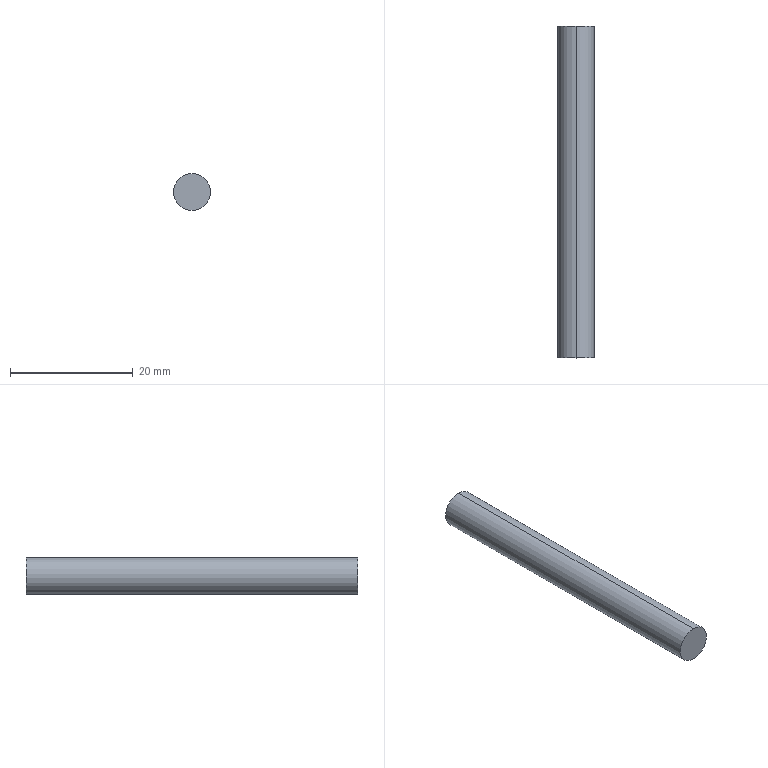Part | STEP file | Hinge shaft | 1 solid | 4 faces | box 6 x 54 x 6 mm | volume 1527 mm3 | cylinder 2 | plane 2 | commonest cylinder face diameters 6 x2
STEP:
#1=CARTESIAN_POINT('',(0.,0.,0.));
#2=DIRECTION('',(0.,0.,1.));
#3=DIRECTION('',(1.,0.,0.));
#4=AXIS2_PLACEMENT_3D('',#1,#2,#3);
#5=CARTESIAN_POINT('',(0.,54.,-3.));
#6=VERTEX_POINT('',#5);
#7=CARTESIAN_POINT('',(0.,54.,3.));
#8=VERTEX_POINT('',#7);
#9=CARTESIAN_POINT('',(0.,54.,0.));
#10=DIRECTION('',(0.,-1.,0.));
#11=DIRECTION('',(0.,0.,-1.));
#12=AXIS2_PLACEMENT_3D('',#9,#10,#11);
#13=CIRCLE('',#12,3.);
#14=CARTESIAN_POINT('',(0.,54.,0.));
#15=DIRECTION('',(0.,-1.,0.));
#16=DIRECTION('',(0.,0.,-1.));
#17=AXIS2_PLACEMENT_3D('',#14,#15,#16);
#18=CYLINDRICAL_SURFACE('',#17,3.);
#19=CARTESIAN_POINT('',(0.,0.));
#20=DIRECTION('',(1.,0.));
#21=VECTOR('',#20,1.);
#22=LINE('',#19,#21);
#23=(GEOMETRIC_REPRESENTATION_CONTEXT(2)PARAMETRIC_REPRESENTATION_CONTEXT()REPRESENTATION_CONTEXT('',''));
#24=DEFINITIONAL_REPRESENTATION('',(#22),#23);
#25=PCURVE('',#18,#24);
#26=CARTESIAN_POINT('',(0.,54.,0.));
#27=DIRECTION('',(0.,1.,0.));
#28=DIRECTION('',(0.,0.,1.));
#29=AXIS2_PLACEMENT_3D('',#26,#27,#28);
#30=PLANE('',#29);
#31=CARTESIAN_POINT('',(-3.,0.));
#32=CARTESIAN_POINT('',(-3.,5.196));
#33=CARTESIAN_POINT('',(1.5,2.598));
#34=CARTESIAN_POINT('',(6.,0.));
#35=CARTESIAN_POINT('',(1.5,-2.598));
#36=CARTESIAN_POINT('',(-3.,-5.196));
#37=CARTESIAN_POINT('',(-3.,0.));
#38=(BOUNDED_CURVE()B_SPLINE_CURVE(2,(#31,#32,#33,#34,#35,#36,#37),.UNSPECIFIED.,.T.,.F.)B_SPLINE_CURVE_WITH_KNOTS((1,2,2,2,2,1),(-2.094,0.,2.094,4.189,6.283,8.378),.UNSPECIFIED.)CURVE()GEOMETRIC_REPRESENTATION_ITEM()RATIONAL_B_SPLINE_CURVE((1.,0.5,1.,0.5,1.,0.5,1.))REPRESENTATION_ITEM(''));
#39=(GEOMETRIC_REPRESENTATION_CONTEXT(2)PARAMETRIC_REPRESENTATION_CONTEXT()REPRESENTATION_CONTEXT('',''));
#40=DEFINITIONAL_REPRESENTATION('',(#38),#39);
#41=PCURVE('',#30,#40);
#42=SURFACE_CURVE('',#13,(#25,#41),.PCURVE_S1.);
#43=EDGE_CURVE('',#6,#8,#42,.T.);
#44=ORIENTED_EDGE('',*,*,#43,.T.);
#45=CARTESIAN_POINT('',(0.,0.,3.));
#46=VERTEX_POINT('',#45);
#47=CARTESIAN_POINT('',(0.,54.,3.));
#48=DIRECTION('',(0.,-1.,0.));
#49=VECTOR('',#48,1.);
#50=LINE('',#47,#49);
#51=CARTESIAN_POINT('',(3.142,0.));
#52=DIRECTION('',(0.,1.));
#53=VECTOR('',#52,1.);
#54=LINE('',#51,#53);
#55=(GEOMETRIC_REPRESENTATION_CONTEXT(2)PARAMETRIC_REPRESENTATION_CONTEXT()REPRESENTATION_CONTEXT('',''));
#56=DEFINITIONAL_REPRESENTATION('',(#54),#55);
#57=PCURVE('',#18,#56);
#58=CARTESIAN_POINT('',(0.,54.,0.));
#59=DIRECTION('',(0.,-1.,0.));
#60=DIRECTION('',(0.,0.,-1.));
#61=AXIS2_PLACEMENT_3D('',#58,#59,#60);
#62=CYLINDRICAL_SURFACE('',#61,3.);
#63=CARTESIAN_POINT('',(3.142,0.));
#64=DIRECTION('',(0.,1.));
#65=VECTOR('',#64,1.);
#66=LINE('',#63,#65);
#67=(GEOMETRIC_REPRESENTATION_CONTEXT(2)PARAMETRIC_REPRESENTATION_CONTEXT()REPRESENTATION_CONTEXT('',''));
#68=DEFINITIONAL_REPRESENTATION('',(#66),#67);
#69=PCURVE('',#62,#68);
#70=SURFACE_CURVE('',#50,(#57,#69),.PCURVE_S1.);
#71=EDGE_CURVE('',#8,#46,#70,.T.);
#72=ORIENTED_EDGE('',*,*,#71,.T.);
#73=CARTESIAN_POINT('',(0.,0.,-3.));
#74=VERTEX_POINT('',#73);
#75=CARTESIAN_POINT('',(0.,0.,0.));
#76=DIRECTION('',(0.,1.,0.));
#77=DIRECTION('',(0.,0.,-1.));
#78=AXIS2_PLACEMENT_3D('',#75,#76,#77);
#79=CIRCLE('',#78,3.);
#80=CARTESIAN_POINT('',(6.283,54.));
#81=DIRECTION('',(-1.,0.));
#82=VECTOR('',#81,1.);
#83=LINE('',#80,#82);
#84=(GEOMETRIC_REPRESENTATION_CONTEXT(2)PARAMETRIC_REPRESENTATION_CONTEXT()REPRESENTATION_CONTEXT('',''));
#85=DEFINITIONAL_REPRESENTATION('',(#83),#84);
#86=PCURVE('',#18,#85);
#87=CARTESIAN_POINT('',(0.,0.,0.));
#88=DIRECTION('',(0.,1.,0.));
#89=DIRECTION('',(0.,0.,1.));
#90=AXIS2_PLACEMENT_3D('',#87,#88,#89);
#91=PLANE('',#90);
#92=CARTESIAN_POINT('',(0.,0.));
#93=DIRECTION('',(-1.,0.));
#94=AXIS2_PLACEMENT_2D('',#92,#93);
#95=CIRCLE('',#94,3.);
#96=(GEOMETRIC_REPRESENTATION_CONTEXT(2)PARAMETRIC_REPRESENTATION_CONTEXT()REPRESENTATION_CONTEXT('',''));
#97=DEFINITIONAL_REPRESENTATION('',(#95),#96);
#98=PCURVE('',#91,#97);
#99=SURFACE_CURVE('',#79,(#86,#98),.PCURVE_S1.);
#100=EDGE_CURVE('',#46,#74,#99,.T.);
#101=ORIENTED_EDGE('',*,*,#100,.T.);
#102=CARTESIAN_POINT('',(0.,54.,-3.));
#103=DIRECTION('',(0.,-1.,0.));
#104=VECTOR('',#103,1.);
#105=LINE('',#102,#104);
#106=CARTESIAN_POINT('',(0.,0.));
#107=DIRECTION('',(0.,1.));
#108=VECTOR('',#107,1.);
#109=LINE('',#106,#108);
#110=(GEOMETRIC_REPRESENTATION_CONTEXT(2)PARAMETRIC_REPRESENTATION_CONTEXT()REPRESENTATION_CONTEXT('',''));
#111=DEFINITIONAL_REPRESENTATION('',(#109),#110);
#112=PCURVE('',#18,#111);
#113=CARTESIAN_POINT('',(6.283,0.));
#114=DIRECTION('',(0.,1.));
#115=VECTOR('',#114,1.);
#116=LINE('',#113,#115);
#117=(GEOMETRIC_REPRESENTATION_CONTEXT(2)PARAMETRIC_REPRESENTATION_CONTEXT()REPRESENTATION_CONTEXT('',''));
#118=DEFINITIONAL_REPRESENTATION('',(#116),#117);
#119=PCURVE('',#62,#118);
#120=SURFACE_CURVE('',#105,(#112,#119),.PCURVE_S1.);
#121=EDGE_CURVE('',#6,#74,#120,.T.);
#122=ORIENTED_EDGE('',*,*,#121,.F.);
#123=EDGE_LOOP('',(#44,#72,#101,#122));
#124=FACE_BOUND('',#123,.T.);
#125=ADVANCED_FACE('',(#124),#18,.T.);
#126=ORIENTED_EDGE('',*,*,#71,.F.);
#127=CARTESIAN_POINT('',(0.,54.,0.));
#128=DIRECTION('',(0.,-1.,0.));
#129=DIRECTION('',(0.,0.,-1.));
#130=AXIS2_PLACEMENT_3D('',#127,#128,#129);
#131=CIRCLE('',#130,3.);
#132=CARTESIAN_POINT('',(0.,0.));
#133=DIRECTION('',(1.,0.));
#134=VECTOR('',#133,1.);
#135=LINE('',#132,#134);
#136=(GEOMETRIC_REPRESENTATION_CONTEXT(2)PARAMETRIC_REPRESENTATION_CONTEXT()REPRESENTATION_CONTEXT('',''));
#137=DEFINITIONAL_REPRESENTATION('',(#135),#136);
#138=PCURVE('',#62,#137);
#139=CARTESIAN_POINT('',(-3.,0.));
#140=CARTESIAN_POINT('',(-3.,5.196));
#141=CARTESIAN_POINT('',(1.5,2.598));
#142=CARTESIAN_POINT('',(6.,0.));
#143=CARTESIAN_POINT('',(1.5,-2.598));
#144=CARTESIAN_POINT('',(-3.,-5.196));
#145=CARTESIAN_POINT('',(-3.,0.));
#146=(BOUNDED_CURVE()B_SPLINE_CURVE(2,(#139,#140,#141,#142,#143,#144,#145),.UNSPECIFIED.,.T.,.F.)B_SPLINE_CURVE_WITH_KNOTS((1,2,2,2,2,1),(-2.094,0.,2.094,4.189,6.283,8.378),.UNSPECIFIED.)CURVE()GEOMETRIC_REPRESENTATION_ITEM()RATIONAL_B_SPLINE_CURVE((1.,0.5,1.,0.5,1.,0.5,1.))REPRESENTATION_ITEM(''));
#147=(GEOMETRIC_REPRESENTATION_CONTEXT(2)PARAMETRIC_REPRESENTATION_CONTEXT()REPRESENTATION_CONTEXT('',''));
#148=DEFINITIONAL_REPRESENTATION('',(#146),#147);
#149=PCURVE('',#30,#148);
#150=SURFACE_CURVE('',#131,(#138,#149),.PCURVE_S1.);
#151=EDGE_CURVE('',#8,#6,#150,.T.);
#152=ORIENTED_EDGE('',*,*,#151,.T.);
#153=ORIENTED_EDGE('',*,*,#121,.T.);
#154=CARTESIAN_POINT('',(0.,0.,0.));
#155=DIRECTION('',(0.,1.,0.));
#156=DIRECTION('',(0.,0.,-1.));
#157=AXIS2_PLACEMENT_3D('',#154,#155,#156);
#158=CIRCLE('',#157,3.);
#159=CARTESIAN_POINT('',(6.283,54.));
#160=DIRECTION('',(-1.,0.));
#161=VECTOR('',#160,1.);
#162=LINE('',#159,#161);
#163=(GEOMETRIC_REPRESENTATION_CONTEXT(2)PARAMETRIC_REPRESENTATION_CONTEXT()REPRESENTATION_CONTEXT('',''));
#164=DEFINITIONAL_REPRESENTATION('',(#162),#163);
#165=PCURVE('',#62,#164);
#166=CARTESIAN_POINT('',(0.,0.));
#167=DIRECTION('',(-1.,0.));
#168=AXIS2_PLACEMENT_2D('',#166,#167);
#169=CIRCLE('',#168,3.);
#170=(GEOMETRIC_REPRESENTATION_CONTEXT(2)PARAMETRIC_REPRESENTATION_CONTEXT()REPRESENTATION_CONTEXT('',''));
#171=DEFINITIONAL_REPRESENTATION('',(#169),#170);
#172=PCURVE('',#91,#171);
#173=SURFACE_CURVE('',#158,(#165,#172),.PCURVE_S1.);
#174=EDGE_CURVE('',#74,#46,#173,.T.);
#175=ORIENTED_EDGE('',*,*,#174,.T.);
#176=EDGE_LOOP('',(#126,#152,#153,#175));
#177=FACE_BOUND('',#176,.T.);
#178=ADVANCED_FACE('',(#177),#62,.T.);
#179=ORIENTED_EDGE('',*,*,#174,.F.);
#180=ORIENTED_EDGE('',*,*,#100,.F.);
#181=EDGE_LOOP('',(#179,#180));
#182=FACE_BOUND('',#181,.T.);
#183=ADVANCED_FACE('',(#182),#91,.F.);
#184=ORIENTED_EDGE('',*,*,#43,.F.);
#185=ORIENTED_EDGE('',*,*,#151,.F.);
#186=EDGE_LOOP('',(#184,#185));
#187=FACE_BOUND('',#186,.T.);
#188=ADVANCED_FACE('',(#187),#30,.T.);
#189=CLOSED_SHELL('',(#125,#178,#183,#188));
#190=MANIFOLD_SOLID_BREP('',#189);
#191=(LENGTH_UNIT()NAMED_UNIT(*)SI_UNIT(.MILLI.,.METRE.));
#192=UNCERTAINTY_MEASURE_WITH_UNIT(LENGTH_MEASURE(0.0000001),#191,'','');
#193=(NAMED_UNIT(*)PLANE_ANGLE_UNIT()SI_UNIT($,.RADIAN.));
#194=(NAMED_UNIT(*)SI_UNIT($,.STERADIAN.)SOLID_ANGLE_UNIT());
#195=(GEOMETRIC_REPRESENTATION_CONTEXT(3)GLOBAL_UNCERTAINTY_ASSIGNED_CONTEXT((#192))GLOBAL_UNIT_ASSIGNED_CONTEXT((#191,#193,#194))REPRESENTATION_CONTEXT('',''));
#196=ADVANCED_BREP_SHAPE_REPRESENTATION('',(#4,#190),#195);